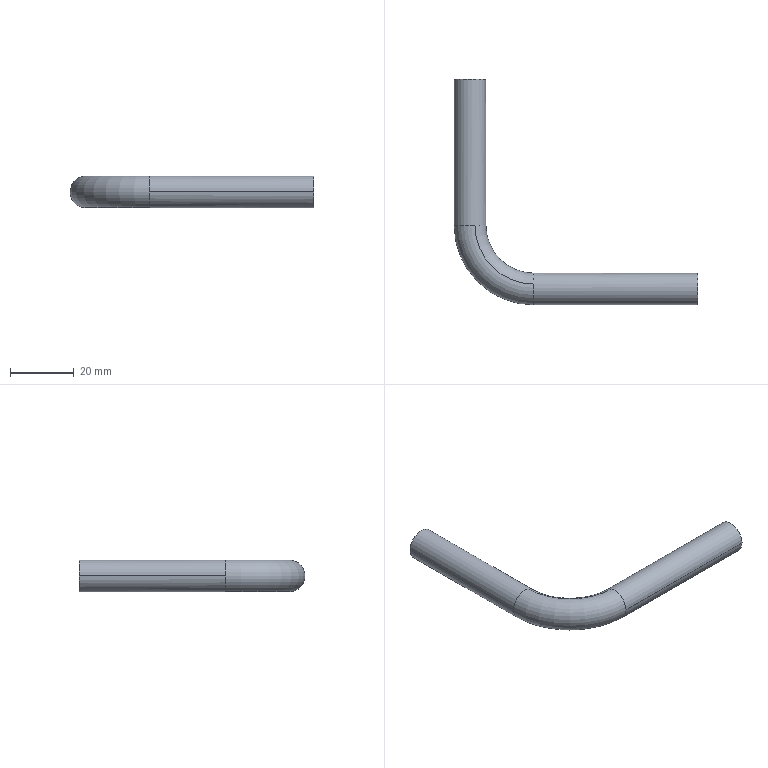Part | 1 solid | 8 faces | box 76.634 x 71 x 10 mm | volume 10136 mm3 | cylinder 4 | plane 2 | torus 2 | commonest cylinder face diameters 10 x4
STEP:
#1=CARTESIAN_POINT('',(0.,0.,0.));
#2=DIRECTION('',(0.,0.,1.));
#3=DIRECTION('',(1.,0.,0.));
#4=AXIS2_PLACEMENT_3D('',#1,#2,#3);
#5=CARTESIAN_POINT('',(-70.758,91.551,-281.55));
#6=VERTEX_POINT('',#5);
#7=CARTESIAN_POINT('',(-70.758,137.551,-281.55));
#8=VERTEX_POINT('',#7);
#9=CARTESIAN_POINT('',(-70.758,91.551,-281.55));
#10=DIRECTION('',(0.,1.,0.));
#11=VECTOR('',#10,1.);
#12=LINE('',#9,#11);
#13=CARTESIAN_POINT('',(-75.758,91.551,-281.55));
#14=DIRECTION('',(0.,1.,0.));
#15=DIRECTION('',(0.,0.,1.));
#16=AXIS2_PLACEMENT_3D('',#13,#14,#15);
#17=CYLINDRICAL_SURFACE('',#16,5.);
#18=CARTESIAN_POINT('',(1.571,0.));
#19=DIRECTION('',(0.,1.));
#20=VECTOR('',#19,1.);
#21=LINE('',#18,#20);
#22=(GEOMETRIC_REPRESENTATION_CONTEXT(2)PARAMETRIC_REPRESENTATION_CONTEXT()REPRESENTATION_CONTEXT('',''));
#23=DEFINITIONAL_REPRESENTATION('',(#21),#22);
#24=PCURVE('',#17,#23);
#25=CARTESIAN_POINT('',(-75.758,91.551,-281.55));
#26=DIRECTION('',(0.,1.,0.));
#27=DIRECTION('',(0.,0.,-1.));
#28=AXIS2_PLACEMENT_3D('',#25,#26,#27);
#29=CYLINDRICAL_SURFACE('',#28,5.);
#30=CARTESIAN_POINT('',(4.712,0.));
#31=DIRECTION('',(0.,1.));
#32=VECTOR('',#31,1.);
#33=LINE('',#30,#32);
#34=(GEOMETRIC_REPRESENTATION_CONTEXT(2)PARAMETRIC_REPRESENTATION_CONTEXT()REPRESENTATION_CONTEXT('',''));
#35=DEFINITIONAL_REPRESENTATION('',(#33),#34);
#36=PCURVE('',#29,#35);
#37=SURFACE_CURVE('',#12,(#24,#36),.PCURVE_S1.);
#38=EDGE_CURVE('',#6,#8,#37,.T.);
#39=ORIENTED_EDGE('',*,*,#38,.F.);
#40=CARTESIAN_POINT('',(-77.304,91.551,-286.305));
#41=VERTEX_POINT('',#40);
#42=CARTESIAN_POINT('',(-75.758,91.551,-281.55));
#43=DIRECTION('',(0.,1.,0.));
#44=DIRECTION('',(-1.,0.,0.));
#45=AXIS2_PLACEMENT_3D('',#42,#43,#44);
#46=CIRCLE('',#45,5.);
#47=CARTESIAN_POINT('',(-1.571,0.));
#48=DIRECTION('',(1.,0.));
#49=VECTOR('',#48,1.);
#50=LINE('',#47,#49);
#51=(GEOMETRIC_REPRESENTATION_CONTEXT(2)PARAMETRIC_REPRESENTATION_CONTEXT()REPRESENTATION_CONTEXT('',''));
#52=DEFINITIONAL_REPRESENTATION('',(#50),#51);
#53=PCURVE('',#17,#52);
#54=CARTESIAN_POINT('',(-55.758,91.551,-281.55));
#55=DIRECTION('',(0.,0.,-1.));
#56=DIRECTION('',(0.7071,0.7071,0.));
#57=AXIS2_PLACEMENT_3D('',#54,#55,#56);
#58=TOROIDAL_SURFACE('',#57,20.,5.);
#59=CARTESIAN_POINT('',(3.927,6.283));
#60=DIRECTION('',(0.,-1.));
#61=VECTOR('',#60,1.);
#62=LINE('',#59,#61);
#63=(GEOMETRIC_REPRESENTATION_CONTEXT(2)PARAMETRIC_REPRESENTATION_CONTEXT()REPRESENTATION_CONTEXT('',''));
#64=DEFINITIONAL_REPRESENTATION('',(#62),#63);
#65=PCURVE('',#58,#64);
#66=SURFACE_CURVE('',#46,(#53,#65),.PCURVE_S1.);
#67=EDGE_CURVE('',#6,#41,#66,.T.);
#68=ORIENTED_EDGE('',*,*,#67,.T.);
#69=CARTESIAN_POINT('',(-80.758,91.551,-281.55));
#70=VERTEX_POINT('',#69);
#71=CARTESIAN_POINT('',(-75.758,91.551,-281.55));
#72=DIRECTION('',(0.,1.,0.));
#73=DIRECTION('',(-1.,0.,0.));
#74=AXIS2_PLACEMENT_3D('',#71,#72,#73);
#75=CIRCLE('',#74,5.);
#76=CARTESIAN_POINT('',(-1.571,0.));
#77=DIRECTION('',(1.,0.));
#78=VECTOR('',#77,1.);
#79=LINE('',#76,#78);
#80=(GEOMETRIC_REPRESENTATION_CONTEXT(2)PARAMETRIC_REPRESENTATION_CONTEXT()REPRESENTATION_CONTEXT('',''));
#81=DEFINITIONAL_REPRESENTATION('',(#79),#80);
#82=PCURVE('',#17,#81);
#83=CARTESIAN_POINT('',(-55.758,91.551,-281.55));
#84=DIRECTION('',(0.,0.,-1.));
#85=DIRECTION('',(0.7071,0.7071,0.));
#86=AXIS2_PLACEMENT_3D('',#83,#84,#85);
#87=TOROIDAL_SURFACE('',#86,20.,5.);
#88=CARTESIAN_POINT('',(3.927,12.566));
#89=DIRECTION('',(0.,-1.));
#90=VECTOR('',#89,1.);
#91=LINE('',#88,#90);
#92=(GEOMETRIC_REPRESENTATION_CONTEXT(2)PARAMETRIC_REPRESENTATION_CONTEXT()REPRESENTATION_CONTEXT('',''));
#93=DEFINITIONAL_REPRESENTATION('',(#91),#92);
#94=PCURVE('',#87,#93);
#95=SURFACE_CURVE('',#75,(#82,#94),.PCURVE_S1.);
#96=EDGE_CURVE('',#41,#70,#95,.T.);
#97=ORIENTED_EDGE('',*,*,#96,.T.);
#98=CARTESIAN_POINT('',(-80.758,137.551,-281.55));
#99=VERTEX_POINT('',#98);
#100=CARTESIAN_POINT('',(-80.758,91.551,-281.55));
#101=DIRECTION('',(0.,1.,0.));
#102=VECTOR('',#101,1.);
#103=LINE('',#100,#102);
#104=CARTESIAN_POINT('',(4.712,0.));
#105=DIRECTION('',(0.,1.));
#106=VECTOR('',#105,1.);
#107=LINE('',#104,#106);
#108=(GEOMETRIC_REPRESENTATION_CONTEXT(2)PARAMETRIC_REPRESENTATION_CONTEXT()REPRESENTATION_CONTEXT('',''));
#109=DEFINITIONAL_REPRESENTATION('',(#107),#108);
#110=PCURVE('',#17,#109);
#111=CARTESIAN_POINT('',(1.571,0.));
#112=DIRECTION('',(0.,1.));
#113=VECTOR('',#112,1.);
#114=LINE('',#111,#113);
#115=(GEOMETRIC_REPRESENTATION_CONTEXT(2)PARAMETRIC_REPRESENTATION_CONTEXT()REPRESENTATION_CONTEXT('',''));
#116=DEFINITIONAL_REPRESENTATION('',(#114),#115);
#117=PCURVE('',#29,#116);
#118=SURFACE_CURVE('',#103,(#110,#117),.PCURVE_S1.);
#119=EDGE_CURVE('',#70,#99,#118,.T.);
#120=ORIENTED_EDGE('',*,*,#119,.T.);
#121=CARTESIAN_POINT('',(-75.758,137.551,-281.55));
#122=DIRECTION('',(0.,1.,0.));
#123=DIRECTION('',(-1.,0.,0.));
#124=AXIS2_PLACEMENT_3D('',#121,#122,#123);
#125=CIRCLE('',#124,5.);
#126=CARTESIAN_POINT('',(-1.571,46.));
#127=DIRECTION('',(1.,0.));
#128=VECTOR('',#127,1.);
#129=LINE('',#126,#128);
#130=(GEOMETRIC_REPRESENTATION_CONTEXT(2)PARAMETRIC_REPRESENTATION_CONTEXT()REPRESENTATION_CONTEXT('',''));
#131=DEFINITIONAL_REPRESENTATION('',(#129),#130);
#132=PCURVE('',#17,#131);
#133=CARTESIAN_POINT('',(-75.758,137.551,-281.55));
#134=DIRECTION('',(0.,1.,0.));
#135=DIRECTION('',(-1.,0.,0.));
#136=AXIS2_PLACEMENT_3D('',#133,#134,#135);
#137=PLANE('',#136);
#138=CARTESIAN_POINT('',(0.,0.));
#139=DIRECTION('',(1.,0.));
#140=AXIS2_PLACEMENT_2D('',#138,#139);
#141=CIRCLE('',#140,5.);
#142=(GEOMETRIC_REPRESENTATION_CONTEXT(2)PARAMETRIC_REPRESENTATION_CONTEXT()REPRESENTATION_CONTEXT('',''));
#143=DEFINITIONAL_REPRESENTATION('',(#141),#142);
#144=PCURVE('',#137,#143);
#145=SURFACE_CURVE('',#125,(#132,#144),.PCURVE_S1.);
#146=EDGE_CURVE('',#8,#99,#145,.T.);
#147=ORIENTED_EDGE('',*,*,#146,.F.);
#148=EDGE_LOOP('',(#39,#68,#97,#120,#147));
#149=FACE_BOUND('',#148,.T.);
#150=ADVANCED_FACE('',(#149),#17,.T.);
#151=CARTESIAN_POINT('',(-75.758,137.551,-281.55));
#152=DIRECTION('',(0.,1.,0.));
#153=DIRECTION('',(-1.,0.,0.));
#154=AXIS2_PLACEMENT_3D('',#151,#152,#153);
#155=CIRCLE('',#154,5.);
#156=CARTESIAN_POINT('',(0.,0.));
#157=DIRECTION('',(1.,0.));
#158=AXIS2_PLACEMENT_2D('',#156,#157);
#159=CIRCLE('',#158,5.);
#160=(GEOMETRIC_REPRESENTATION_CONTEXT(2)PARAMETRIC_REPRESENTATION_CONTEXT()REPRESENTATION_CONTEXT('',''));
#161=DEFINITIONAL_REPRESENTATION('',(#159),#160);
#162=PCURVE('',#137,#161);
#163=CARTESIAN_POINT('',(1.571,46.));
#164=DIRECTION('',(1.,0.));
#165=VECTOR('',#164,1.);
#166=LINE('',#163,#165);
#167=(GEOMETRIC_REPRESENTATION_CONTEXT(2)PARAMETRIC_REPRESENTATION_CONTEXT()REPRESENTATION_CONTEXT('',''));
#168=DEFINITIONAL_REPRESENTATION('',(#166),#167);
#169=PCURVE('',#29,#168);
#170=SURFACE_CURVE('',#155,(#162,#169),.PCURVE_S1.);
#171=EDGE_CURVE('',#99,#8,#170,.T.);
#172=ORIENTED_EDGE('',*,*,#171,.T.);
#173=ORIENTED_EDGE('',*,*,#146,.T.);
#174=EDGE_LOOP('',(#172,#173));
#175=FACE_BOUND('',#174,.T.);
#176=ADVANCED_FACE('',(#175),#137,.T.);
#177=CARTESIAN_POINT('',(-55.758,73.096,-276.795));
#178=VERTEX_POINT('',#177);
#179=CARTESIAN_POINT('',(-74.213,91.551,-276.795));
#180=VERTEX_POINT('',#179);
#181=CARTESIAN_POINT('',(-55.758,91.551,-276.795));
#182=DIRECTION('',(0.,0.,-1.));
#183=DIRECTION('',(0.,-1.,0.));
#184=AXIS2_PLACEMENT_3D('',#181,#182,#183);
#185=CIRCLE('',#184,18.455);
#186=CARTESIAN_POINT('',(2.356,4.398));
#187=DIRECTION('',(1.,0.));
#188=VECTOR('',#187,1.);
#189=LINE('',#186,#188);
#190=(GEOMETRIC_REPRESENTATION_CONTEXT(2)PARAMETRIC_REPRESENTATION_CONTEXT()REPRESENTATION_CONTEXT('',''));
#191=DEFINITIONAL_REPRESENTATION('',(#189),#190);
#192=PCURVE('',#58,#191);
#193=CARTESIAN_POINT('',(2.356,4.398));
#194=DIRECTION('',(1.,0.));
#195=VECTOR('',#194,1.);
#196=LINE('',#193,#195);
#197=(GEOMETRIC_REPRESENTATION_CONTEXT(2)PARAMETRIC_REPRESENTATION_CONTEXT()REPRESENTATION_CONTEXT('',''));
#198=DEFINITIONAL_REPRESENTATION('',(#196),#197);
#199=PCURVE('',#87,#198);
#200=SURFACE_CURVE('',#185,(#192,#199),.PCURVE_S1.);
#201=EDGE_CURVE('',#178,#180,#200,.T.);
#202=ORIENTED_EDGE('',*,*,#201,.F.);
#203=CARTESIAN_POINT('',(-55.758,76.551,-281.55));
#204=VERTEX_POINT('',#203);
#205=CARTESIAN_POINT('',(-55.758,71.551,-281.55));
#206=DIRECTION('',(-1.,0.,0.));
#207=DIRECTION('',(0.,1.,0.));
#208=AXIS2_PLACEMENT_3D('',#205,#206,#207);
#209=CIRCLE('',#208,5.);
#210=CARTESIAN_POINT('',(2.356,9.425));
#211=DIRECTION('',(0.,-1.));
#212=VECTOR('',#211,1.);
#213=LINE('',#210,#212);
#214=(GEOMETRIC_REPRESENTATION_CONTEXT(2)PARAMETRIC_REPRESENTATION_CONTEXT()REPRESENTATION_CONTEXT('',''));
#215=DEFINITIONAL_REPRESENTATION('',(#213),#214);
#216=PCURVE('',#58,#215);
#217=CARTESIAN_POINT('',(-55.758,71.551,-281.55));
#218=DIRECTION('',(1.,0.,0.));
#219=DIRECTION('',(0.,0.,-1.));
#220=AXIS2_PLACEMENT_3D('',#217,#218,#219);
#221=CYLINDRICAL_SURFACE('',#220,5.);
#222=CARTESIAN_POINT('',(7.854,0.));
#223=DIRECTION('',(-1.,0.));
#224=VECTOR('',#223,1.);
#225=LINE('',#222,#224);
#226=(GEOMETRIC_REPRESENTATION_CONTEXT(2)PARAMETRIC_REPRESENTATION_CONTEXT()REPRESENTATION_CONTEXT('',''));
#227=DEFINITIONAL_REPRESENTATION('',(#225),#226);
#228=PCURVE('',#221,#227);
#229=SURFACE_CURVE('',#209,(#216,#228),.PCURVE_S1.);
#230=EDGE_CURVE('',#178,#204,#229,.T.);
#231=ORIENTED_EDGE('',*,*,#230,.T.);
#232=CARTESIAN_POINT('',(-55.758,70.006,-286.305));
#233=VERTEX_POINT('',#232);
#234=CARTESIAN_POINT('',(-55.758,71.551,-281.55));
#235=DIRECTION('',(-1.,0.,0.));
#236=DIRECTION('',(0.,1.,0.));
#237=AXIS2_PLACEMENT_3D('',#234,#235,#236);
#238=CIRCLE('',#237,5.);
#239=CARTESIAN_POINT('',(2.356,3.142));
#240=DIRECTION('',(0.,-1.));
#241=VECTOR('',#240,1.);
#242=LINE('',#239,#241);
#243=(GEOMETRIC_REPRESENTATION_CONTEXT(2)PARAMETRIC_REPRESENTATION_CONTEXT()REPRESENTATION_CONTEXT('',''));
#244=DEFINITIONAL_REPRESENTATION('',(#242),#243);
#245=PCURVE('',#58,#244);
#246=CARTESIAN_POINT('',(-55.758,71.551,-281.55));
#247=DIRECTION('',(1.,0.,0.));
#248=DIRECTION('',(0.,0.,1.));
#249=AXIS2_PLACEMENT_3D('',#246,#247,#248);
#250=CYLINDRICAL_SURFACE('',#249,5.);
#251=CARTESIAN_POINT('',(4.712,0.));
#252=DIRECTION('',(-1.,0.));
#253=VECTOR('',#252,1.);
#254=LINE('',#251,#253);
#255=(GEOMETRIC_REPRESENTATION_CONTEXT(2)PARAMETRIC_REPRESENTATION_CONTEXT()REPRESENTATION_CONTEXT('',''));
#256=DEFINITIONAL_REPRESENTATION('',(#254),#255);
#257=PCURVE('',#250,#256);
#258=SURFACE_CURVE('',#238,(#245,#257),.PCURVE_S1.);
#259=EDGE_CURVE('',#204,#233,#258,.T.);
#260=ORIENTED_EDGE('',*,*,#259,.T.);
#261=CARTESIAN_POINT('',(-55.758,91.551,-286.305));
#262=DIRECTION('',(0.,0.,-1.));
#263=DIRECTION('',(0.,-1.,0.));
#264=AXIS2_PLACEMENT_3D('',#261,#262,#263);
#265=CIRCLE('',#264,21.545);
#266=CARTESIAN_POINT('',(2.356,1.257));
#267=DIRECTION('',(1.,0.));
#268=VECTOR('',#267,1.);
#269=LINE('',#266,#268);
#270=(GEOMETRIC_REPRESENTATION_CONTEXT(2)PARAMETRIC_REPRESENTATION_CONTEXT()REPRESENTATION_CONTEXT('',''));
#271=DEFINITIONAL_REPRESENTATION('',(#269),#270);
#272=PCURVE('',#58,#271);
#273=CARTESIAN_POINT('',(2.356,7.54));
#274=DIRECTION('',(1.,0.));
#275=VECTOR('',#274,1.);
#276=LINE('',#273,#275);
#277=(GEOMETRIC_REPRESENTATION_CONTEXT(2)PARAMETRIC_REPRESENTATION_CONTEXT()REPRESENTATION_CONTEXT('',''));
#278=DEFINITIONAL_REPRESENTATION('',(#276),#277);
#279=PCURVE('',#87,#278);
#280=SURFACE_CURVE('',#265,(#272,#279),.PCURVE_S1.);
#281=EDGE_CURVE('',#233,#41,#280,.T.);
#282=ORIENTED_EDGE('',*,*,#281,.T.);
#283=ORIENTED_EDGE('',*,*,#67,.F.);
#284=CARTESIAN_POINT('',(-75.758,91.551,-281.55));
#285=DIRECTION('',(0.,1.,0.));
#286=DIRECTION('',(-1.,0.,0.));
#287=AXIS2_PLACEMENT_3D('',#284,#285,#286);
#288=CIRCLE('',#287,5.);
#289=CARTESIAN_POINT('',(3.927,6.283));
#290=DIRECTION('',(0.,-1.));
#291=VECTOR('',#290,1.);
#292=LINE('',#289,#291);
#293=(GEOMETRIC_REPRESENTATION_CONTEXT(2)PARAMETRIC_REPRESENTATION_CONTEXT()REPRESENTATION_CONTEXT('',''));
#294=DEFINITIONAL_REPRESENTATION('',(#292),#293);
#295=PCURVE('',#58,#294);
#296=CARTESIAN_POINT('',(1.571,0.));
#297=DIRECTION('',(1.,0.));
#298=VECTOR('',#297,1.);
#299=LINE('',#296,#298);
#300=(GEOMETRIC_REPRESENTATION_CONTEXT(2)PARAMETRIC_REPRESENTATION_CONTEXT()REPRESENTATION_CONTEXT('',''));
#301=DEFINITIONAL_REPRESENTATION('',(#299),#300);
#302=PCURVE('',#29,#301);
#303=SURFACE_CURVE('',#288,(#295,#302),.PCURVE_S1.);
#304=EDGE_CURVE('',#180,#6,#303,.T.);
#305=ORIENTED_EDGE('',*,*,#304,.F.);
#306=EDGE_LOOP('',(#202,#231,#260,#282,#283,#305));
#307=FACE_BOUND('',#306,.T.);
#308=ADVANCED_FACE('',(#307),#58,.T.);
#309=CARTESIAN_POINT('',(-55.758,66.551,-281.55));
#310=VERTEX_POINT('',#309);
#311=CARTESIAN_POINT('',(-4.124,66.551,-281.55));
#312=VERTEX_POINT('',#311);
#313=CARTESIAN_POINT('',(-55.758,66.551,-281.55));
#314=DIRECTION('',(1.,0.,0.));
#315=VECTOR('',#314,1.);
#316=LINE('',#313,#315);
#317=CARTESIAN_POINT('',(1.571,0.));
#318=DIRECTION('',(0.,1.));
#319=VECTOR('',#318,1.);
#320=LINE('',#317,#319);
#321=(GEOMETRIC_REPRESENTATION_CONTEXT(2)PARAMETRIC_REPRESENTATION_CONTEXT()REPRESENTATION_CONTEXT('',''));
#322=DEFINITIONAL_REPRESENTATION('',(#320),#321);
#323=PCURVE('',#250,#322);
#324=CARTESIAN_POINT('',(4.712,0.));
#325=DIRECTION('',(0.,1.));
#326=VECTOR('',#325,1.);
#327=LINE('',#324,#326);
#328=(GEOMETRIC_REPRESENTATION_CONTEXT(2)PARAMETRIC_REPRESENTATION_CONTEXT()REPRESENTATION_CONTEXT('',''));
#329=DEFINITIONAL_REPRESENTATION('',(#327),#328);
#330=PCURVE('',#221,#329);
#331=SURFACE_CURVE('',#316,(#323,#330),.PCURVE_S1.);
#332=EDGE_CURVE('',#310,#312,#331,.T.);
#333=ORIENTED_EDGE('',*,*,#332,.F.);
#334=CARTESIAN_POINT('',(-55.758,71.551,-281.55));
#335=DIRECTION('',(-1.,0.,0.));
#336=DIRECTION('',(0.,1.,0.));
#337=AXIS2_PLACEMENT_3D('',#334,#335,#336);
#338=CIRCLE('',#337,5.);
#339=CARTESIAN_POINT('',(4.712,0.));
#340=DIRECTION('',(-1.,0.));
#341=VECTOR('',#340,1.);
#342=LINE('',#339,#341);
#343=(GEOMETRIC_REPRESENTATION_CONTEXT(2)PARAMETRIC_REPRESENTATION_CONTEXT()REPRESENTATION_CONTEXT('',''));
#344=DEFINITIONAL_REPRESENTATION('',(#342),#343);
#345=PCURVE('',#250,#344);
#346=CARTESIAN_POINT('',(2.356,9.425));
#347=DIRECTION('',(0.,-1.));
#348=VECTOR('',#347,1.);
#349=LINE('',#346,#348);
#350=(GEOMETRIC_REPRESENTATION_CONTEXT(2)PARAMETRIC_REPRESENTATION_CONTEXT()REPRESENTATION_CONTEXT('',''));
#351=DEFINITIONAL_REPRESENTATION('',(#349),#350);
#352=PCURVE('',#87,#351);
#353=SURFACE_CURVE('',#338,(#345,#352),.PCURVE_S1.);
#354=EDGE_CURVE('',#233,#310,#353,.T.);
#355=ORIENTED_EDGE('',*,*,#354,.F.);
#356=ORIENTED_EDGE('',*,*,#259,.F.);
#357=CARTESIAN_POINT('',(-4.124,76.551,-281.55));
#358=VERTEX_POINT('',#357);
#359=CARTESIAN_POINT('',(-55.758,76.551,-281.55));
#360=DIRECTION('',(1.,0.,0.));
#361=VECTOR('',#360,1.);
#362=LINE('',#359,#361);
#363=CARTESIAN_POINT('',(4.712,0.));
#364=DIRECTION('',(0.,1.));
#365=VECTOR('',#364,1.);
#366=LINE('',#363,#365);
#367=(GEOMETRIC_REPRESENTATION_CONTEXT(2)PARAMETRIC_REPRESENTATION_CONTEXT()REPRESENTATION_CONTEXT('',''));
#368=DEFINITIONAL_REPRESENTATION('',(#366),#367);
#369=PCURVE('',#250,#368);
#370=CARTESIAN_POINT('',(1.571,0.));
#371=DIRECTION('',(0.,1.));
#372=VECTOR('',#371,1.);
#373=LINE('',#370,#372);
#374=(GEOMETRIC_REPRESENTATION_CONTEXT(2)PARAMETRIC_REPRESENTATION_CONTEXT()REPRESENTATION_CONTEXT('',''));
#375=DEFINITIONAL_REPRESENTATION('',(#373),#374);
#376=PCURVE('',#221,#375);
#377=SURFACE_CURVE('',#362,(#369,#376),.PCURVE_S1.);
#378=EDGE_CURVE('',#204,#358,#377,.T.);
#379=ORIENTED_EDGE('',*,*,#378,.T.);
#380=CARTESIAN_POINT('',(-4.124,71.551,-281.55));
#381=DIRECTION('',(-1.,0.,0.));
#382=DIRECTION('',(0.,1.,0.));
#383=AXIS2_PLACEMENT_3D('',#380,#381,#382);
#384=CIRCLE('',#383,5.);
#385=CARTESIAN_POINT('',(4.712,51.634));
#386=DIRECTION('',(-1.,0.));
#387=VECTOR('',#386,1.);
#388=LINE('',#385,#387);
#389=(GEOMETRIC_REPRESENTATION_CONTEXT(2)PARAMETRIC_REPRESENTATION_CONTEXT()REPRESENTATION_CONTEXT('',''));
#390=DEFINITIONAL_REPRESENTATION('',(#388),#389);
#391=PCURVE('',#250,#390);
#392=CARTESIAN_POINT('',(-4.124,71.551,-281.55));
#393=DIRECTION('',(-1.,0.,0.));
#394=DIRECTION('',(0.,-1.,0.));
#395=AXIS2_PLACEMENT_3D('',#392,#393,#394);
#396=PLANE('',#395);
#397=CARTESIAN_POINT('',(0.,0.));
#398=DIRECTION('',(-1.,0.));
#399=AXIS2_PLACEMENT_2D('',#397,#398);
#400=CIRCLE('',#399,5.);
#401=(GEOMETRIC_REPRESENTATION_CONTEXT(2)PARAMETRIC_REPRESENTATION_CONTEXT()REPRESENTATION_CONTEXT('',''));
#402=DEFINITIONAL_REPRESENTATION('',(#400),#401);
#403=PCURVE('',#396,#402);
#404=SURFACE_CURVE('',#384,(#391,#403),.PCURVE_S1.);
#405=EDGE_CURVE('',#358,#312,#404,.T.);
#406=ORIENTED_EDGE('',*,*,#405,.T.);
#407=EDGE_LOOP('',(#333,#355,#356,#379,#406));
#408=FACE_BOUND('',#407,.T.);
#409=ADVANCED_FACE('',(#408),#250,.T.);
#410=CARTESIAN_POINT('',(-4.124,71.551,-281.55));
#411=DIRECTION('',(-1.,0.,0.));
#412=DIRECTION('',(0.,1.,0.));
#413=AXIS2_PLACEMENT_3D('',#410,#411,#412);
#414=CIRCLE('',#413,5.);
#415=CARTESIAN_POINT('',(0.,0.));
#416=DIRECTION('',(-1.,0.));
#417=AXIS2_PLACEMENT_2D('',#415,#416);
#418=CIRCLE('',#417,5.);
#419=(GEOMETRIC_REPRESENTATION_CONTEXT(2)PARAMETRIC_REPRESENTATION_CONTEXT()REPRESENTATION_CONTEXT('',''));
#420=DEFINITIONAL_REPRESENTATION('',(#418),#419);
#421=PCURVE('',#396,#420);
#422=CARTESIAN_POINT('',(7.854,51.634));
#423=DIRECTION('',(-1.,0.));
#424=VECTOR('',#423,1.);
#425=LINE('',#422,#424);
#426=(GEOMETRIC_REPRESENTATION_CONTEXT(2)PARAMETRIC_REPRESENTATION_CONTEXT()REPRESENTATION_CONTEXT('',''));
#427=DEFINITIONAL_REPRESENTATION('',(#425),#426);
#428=PCURVE('',#221,#427);
#429=SURFACE_CURVE('',#414,(#421,#428),.PCURVE_S1.);
#430=EDGE_CURVE('',#312,#358,#429,.T.);
#431=ORIENTED_EDGE('',*,*,#430,.F.);
#432=ORIENTED_EDGE('',*,*,#405,.F.);
#433=EDGE_LOOP('',(#431,#432));
#434=FACE_BOUND('',#433,.T.);
#435=ADVANCED_FACE('',(#434),#396,.F.);
#436=ORIENTED_EDGE('',*,*,#38,.T.);
#437=ORIENTED_EDGE('',*,*,#171,.F.);
#438=ORIENTED_EDGE('',*,*,#119,.F.);
#439=CARTESIAN_POINT('',(-75.758,91.551,-281.55));
#440=DIRECTION('',(0.,1.,0.));
#441=DIRECTION('',(-1.,0.,0.));
#442=AXIS2_PLACEMENT_3D('',#439,#440,#441);
#443=CIRCLE('',#442,5.);
#444=CARTESIAN_POINT('',(1.571,0.));
#445=DIRECTION('',(1.,0.));
#446=VECTOR('',#445,1.);
#447=LINE('',#444,#446);
#448=(GEOMETRIC_REPRESENTATION_CONTEXT(2)PARAMETRIC_REPRESENTATION_CONTEXT()REPRESENTATION_CONTEXT('',''));
#449=DEFINITIONAL_REPRESENTATION('',(#447),#448);
#450=PCURVE('',#29,#449);
#451=CARTESIAN_POINT('',(3.927,6.283));
#452=DIRECTION('',(0.,-1.));
#453=VECTOR('',#452,1.);
#454=LINE('',#451,#453);
#455=(GEOMETRIC_REPRESENTATION_CONTEXT(2)PARAMETRIC_REPRESENTATION_CONTEXT()REPRESENTATION_CONTEXT('',''));
#456=DEFINITIONAL_REPRESENTATION('',(#454),#455);
#457=PCURVE('',#87,#456);
#458=SURFACE_CURVE('',#443,(#450,#457),.PCURVE_S1.);
#459=EDGE_CURVE('',#70,#180,#458,.T.);
#460=ORIENTED_EDGE('',*,*,#459,.T.);
#461=ORIENTED_EDGE('',*,*,#304,.T.);
#462=EDGE_LOOP('',(#436,#437,#438,#460,#461));
#463=FACE_BOUND('',#462,.T.);
#464=ADVANCED_FACE('',(#463),#29,.T.);
#465=ORIENTED_EDGE('',*,*,#201,.T.);
#466=ORIENTED_EDGE('',*,*,#459,.F.);
#467=ORIENTED_EDGE('',*,*,#96,.F.);
#468=ORIENTED_EDGE('',*,*,#281,.F.);
#469=ORIENTED_EDGE('',*,*,#354,.T.);
#470=CARTESIAN_POINT('',(-55.758,71.551,-281.55));
#471=DIRECTION('',(-1.,0.,0.));
#472=DIRECTION('',(0.,1.,0.));
#473=AXIS2_PLACEMENT_3D('',#470,#471,#472);
#474=CIRCLE('',#473,5.);
#475=CARTESIAN_POINT('',(2.356,9.425));
#476=DIRECTION('',(0.,-1.));
#477=VECTOR('',#476,1.);
#478=LINE('',#475,#477);
#479=(GEOMETRIC_REPRESENTATION_CONTEXT(2)PARAMETRIC_REPRESENTATION_CONTEXT()REPRESENTATION_CONTEXT('',''));
#480=DEFINITIONAL_REPRESENTATION('',(#478),#479);
#481=PCURVE('',#87,#480);
#482=CARTESIAN_POINT('',(7.854,0.));
#483=DIRECTION('',(-1.,0.));
#484=VECTOR('',#483,1.);
#485=LINE('',#482,#484);
#486=(GEOMETRIC_REPRESENTATION_CONTEXT(2)PARAMETRIC_REPRESENTATION_CONTEXT()REPRESENTATION_CONTEXT('',''));
#487=DEFINITIONAL_REPRESENTATION('',(#485),#486);
#488=PCURVE('',#221,#487);
#489=SURFACE_CURVE('',#474,(#481,#488),.PCURVE_S1.);
#490=EDGE_CURVE('',#310,#178,#489,.T.);
#491=ORIENTED_EDGE('',*,*,#490,.T.);
#492=EDGE_LOOP('',(#465,#466,#467,#468,#469,#491));
#493=FACE_BOUND('',#492,.T.);
#494=ADVANCED_FACE('',(#493),#87,.T.);
#495=ORIENTED_EDGE('',*,*,#332,.T.);
#496=ORIENTED_EDGE('',*,*,#430,.T.);
#497=ORIENTED_EDGE('',*,*,#378,.F.);
#498=ORIENTED_EDGE('',*,*,#230,.F.);
#499=ORIENTED_EDGE('',*,*,#490,.F.);
#500=EDGE_LOOP('',(#495,#496,#497,#498,#499));
#501=FACE_BOUND('',#500,.T.);
#502=ADVANCED_FACE('',(#501),#221,.T.);
#503=CLOSED_SHELL('',(#150,#176,#308,#409,#435,#464,#494,#502));
#504=MANIFOLD_SOLID_BREP('',#503);
#505=(LENGTH_UNIT()NAMED_UNIT(*)SI_UNIT(.MILLI.,.METRE.));
#506=UNCERTAINTY_MEASURE_WITH_UNIT(LENGTH_MEASURE(0.0000001),#505,'','');
#507=(NAMED_UNIT(*)PLANE_ANGLE_UNIT()SI_UNIT($,.RADIAN.));
#508=(NAMED_UNIT(*)SI_UNIT($,.STERADIAN.)SOLID_ANGLE_UNIT());
#509=(GEOMETRIC_REPRESENTATION_CONTEXT(3)GLOBAL_UNCERTAINTY_ASSIGNED_CONTEXT((#506))GLOBAL_UNIT_ASSIGNED_CONTEXT((#505,#507,#508))REPRESENTATION_CONTEXT('',''));
#510=ADVANCED_BREP_SHAPE_REPRESENTATION('',(#4,#504),#509);